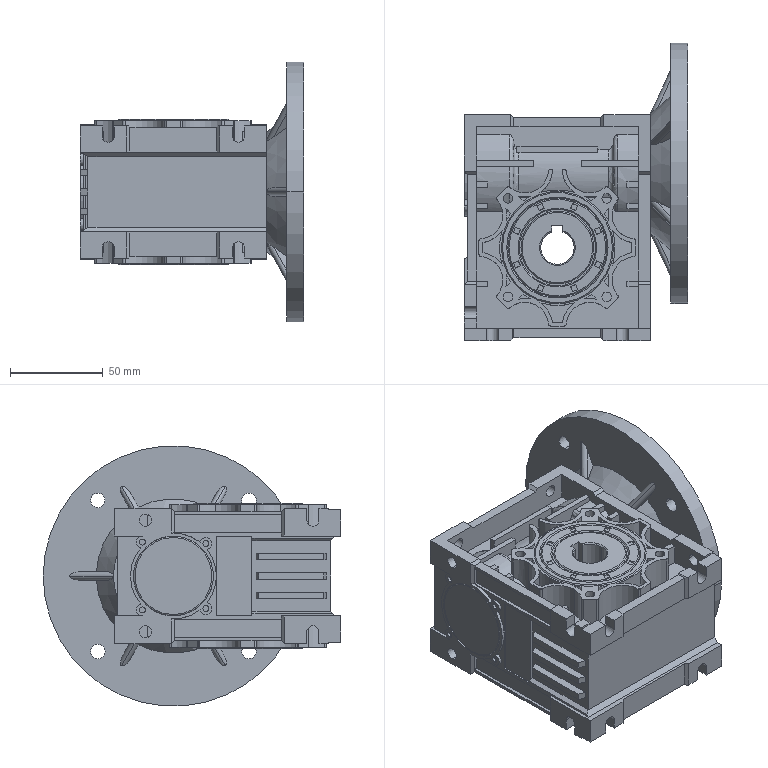Part | STEP file | RV series aluminium alloy worm gear reducer RV40-63 | 1 solid | 778 faces | box 120 x 160 x 140 mm | volume 864960 mm3 | plane 455 | cylinder 257 | torus 38 | cone 28 | commonest cylinder face diameters 2.106 x42 29.795 x36 6.5 x28 62.25 x26 25.583 x20 59.75 x20